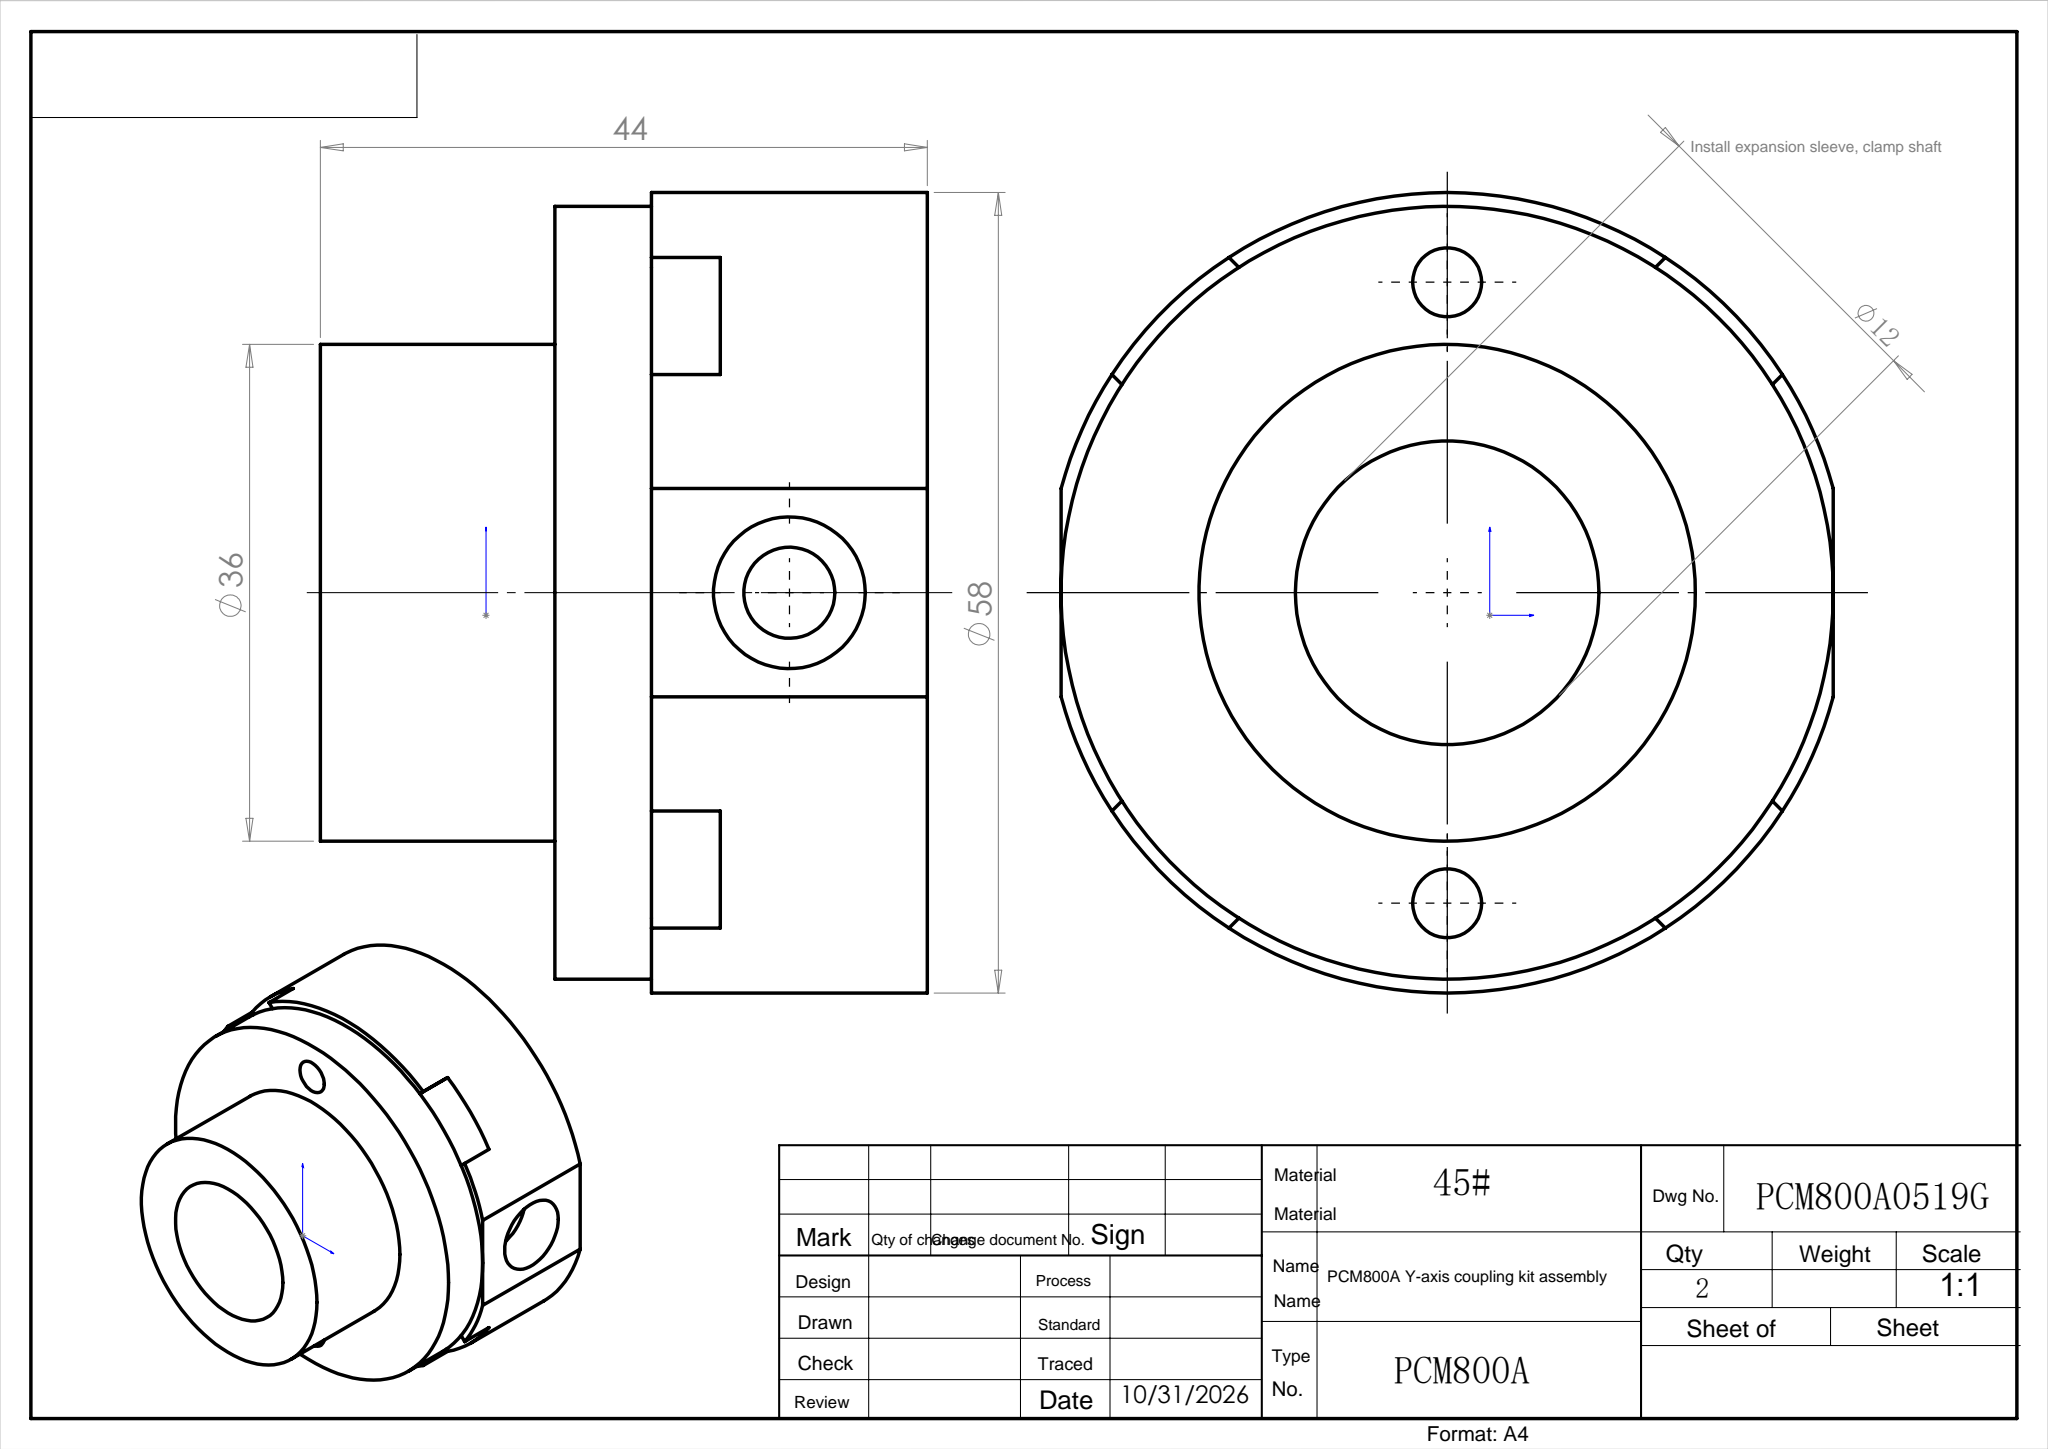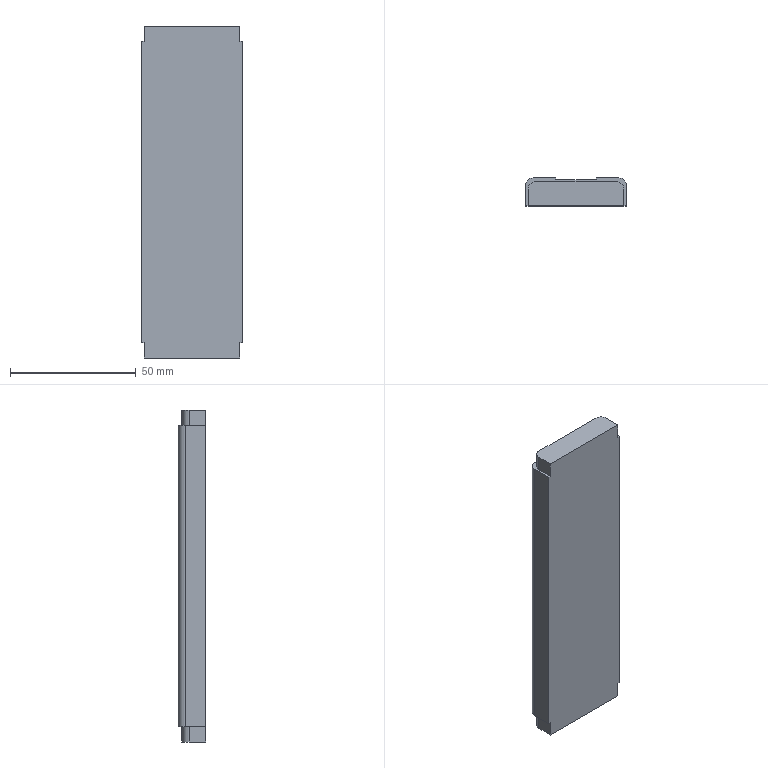Part | SolidWorks | features Boss 2, Cut 2, Extrusion 1 | 1 solid | 48 faces | box 40 x 11 x 132 mm | volume 53803 mm3 | plane 26 | cylinder 22 | commonest cylinder face diameters 5 x16 6 x6